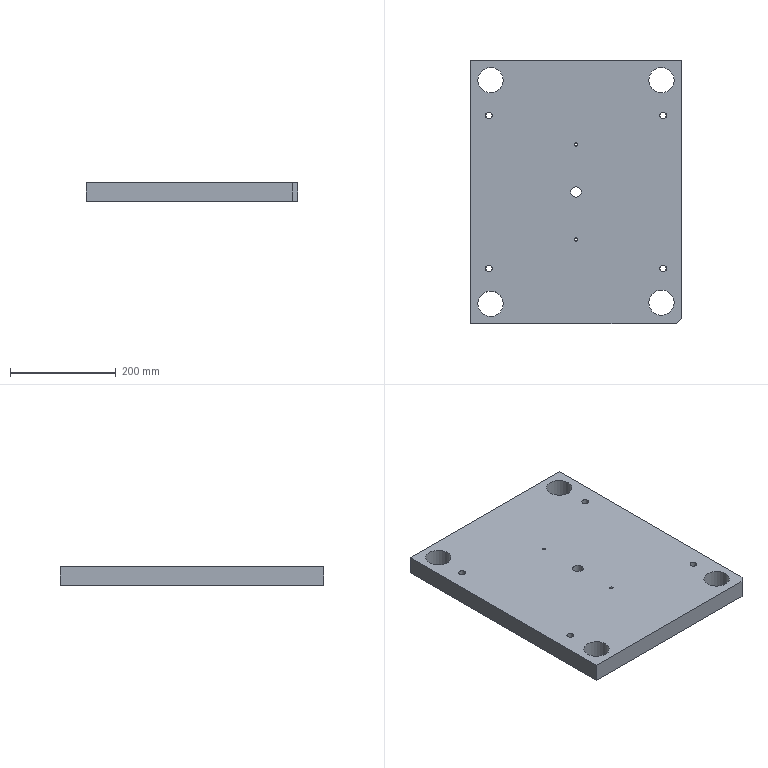Part | STEP file | SL2-MOLD_id726_xmt_txt | 1 solid | 28 faces | box 400 x 500 x 35 mm | volume 6713866 mm3 | cylinder 15 | plane 11 | cone 2 | commonest cylinder face diameters 12 x4 13 x4 48 x4 6 x2 20 x1
STEP:
#1=CARTESIAN_POINT('',(-171.,235.,109.));
#2=VERTEX_POINT('',#1);
#3=CARTESIAN_POINT('',(-165.,235.,109.));
#4=DIRECTION('',(0.,0.,1.));
#5=DIRECTION('',(-1.,0.,0.));
#6=AXIS2_PLACEMENT_3D('',#3,#4,#5);
#7=CIRCLE('',#6,6.);
#8=EDGE_CURVE('',#2,#2,#7,.T.);
#9=ORIENTED_EDGE('',*,*,#8,.F.);
#10=EDGE_LOOP('',(#9));
#11=FACE_BOUND('',#10,.T.);
#12=CARTESIAN_POINT('',(-171.5,235.,109.));
#13=VERTEX_POINT('',#12);
#14=CARTESIAN_POINT('',(-165.,235.,109.));
#15=DIRECTION('',(0.,0.,-1.));
#16=DIRECTION('',(-1.,0.,0.));
#17=AXIS2_PLACEMENT_3D('',#14,#15,#16);
#18=CIRCLE('',#17,6.5);
#19=EDGE_CURVE('',#13,#13,#18,.T.);
#20=ORIENTED_EDGE('',*,*,#19,.F.);
#21=EDGE_LOOP('',(#20));
#22=FACE_BOUND('',#21,.T.);
#23=CARTESIAN_POINT('',(0.,90.,109.));
#24=DIRECTION('',(0.,0.,-1.));
#25=DIRECTION('',(-1.,0.,0.));
#26=AXIS2_PLACEMENT_3D('',#23,#24,#25);
#27=PLANE('',#26);
#28=ADVANCED_FACE('',(#11,#22),#27,.F.);
#29=CARTESIAN_POINT('',(-171.5,-55.,109.));
#30=VERTEX_POINT('',#29);
#31=CARTESIAN_POINT('',(-165.,-55.,109.));
#32=DIRECTION('',(0.,0.,1.));
#33=DIRECTION('',(-1.,0.,0.));
#34=AXIS2_PLACEMENT_3D('',#31,#32,#33);
#35=CIRCLE('',#34,6.5);
#36=EDGE_CURVE('',#30,#30,#35,.T.);
#37=ORIENTED_EDGE('',*,*,#36,.T.);
#38=EDGE_LOOP('',(#37));
#39=FACE_BOUND('',#38,.T.);
#40=CARTESIAN_POINT('',(-171.,-55.,109.));
#41=VERTEX_POINT('',#40);
#42=CARTESIAN_POINT('',(-165.,-55.,109.));
#43=DIRECTION('',(0.,0.,-1.));
#44=DIRECTION('',(-1.,0.,0.));
#45=AXIS2_PLACEMENT_3D('',#42,#43,#44);
#46=CIRCLE('',#45,6.);
#47=EDGE_CURVE('',#41,#41,#46,.T.);
#48=ORIENTED_EDGE('',*,*,#47,.T.);
#49=EDGE_LOOP('',(#48));
#50=FACE_BOUND('',#49,.T.);
#51=CARTESIAN_POINT('',(0.,90.,109.));
#52=DIRECTION('',(0.,0.,-1.));
#53=DIRECTION('',(-1.,0.,0.));
#54=AXIS2_PLACEMENT_3D('',#51,#52,#53);
#55=PLANE('',#54);
#56=ADVANCED_FACE('',(#39,#50),#55,.F.);
#57=CARTESIAN_POINT('',(159.,-55.,109.));
#58=VERTEX_POINT('',#57);
#59=CARTESIAN_POINT('',(165.,-55.,109.));
#60=DIRECTION('',(0.,0.,1.));
#61=DIRECTION('',(-1.,0.,0.));
#62=AXIS2_PLACEMENT_3D('',#59,#60,#61);
#63=CIRCLE('',#62,6.);
#64=EDGE_CURVE('',#58,#58,#63,.T.);
#65=ORIENTED_EDGE('',*,*,#64,.F.);
#66=EDGE_LOOP('',(#65));
#67=FACE_BOUND('',#66,.T.);
#68=CARTESIAN_POINT('',(158.5,-55.,109.));
#69=VERTEX_POINT('',#68);
#70=CARTESIAN_POINT('',(165.,-55.,109.));
#71=DIRECTION('',(0.,0.,-1.));
#72=DIRECTION('',(-1.,0.,0.));
#73=AXIS2_PLACEMENT_3D('',#70,#71,#72);
#74=CIRCLE('',#73,6.5);
#75=EDGE_CURVE('',#69,#69,#74,.T.);
#76=ORIENTED_EDGE('',*,*,#75,.F.);
#77=EDGE_LOOP('',(#76));
#78=FACE_BOUND('',#77,.T.);
#79=CARTESIAN_POINT('',(0.,90.,109.));
#80=DIRECTION('',(0.,0.,-1.));
#81=DIRECTION('',(-1.,0.,0.));
#82=AXIS2_PLACEMENT_3D('',#79,#80,#81);
#83=PLANE('',#82);
#84=ADVANCED_FACE('',(#67,#78),#83,.F.);
#85=CARTESIAN_POINT('',(-159.,235.,101.));
#86=VERTEX_POINT('',#85);
#87=CARTESIAN_POINT('',(-165.,235.,101.));
#88=DIRECTION('',(0.,0.,1.));
#89=DIRECTION('',(1.,0.,0.));
#90=AXIS2_PLACEMENT_3D('',#87,#88,#89);
#91=CIRCLE('',#90,6.);
#92=EDGE_CURVE('',#86,#86,#91,.T.);
#93=ORIENTED_EDGE('',*,*,#92,.T.);
#94=EDGE_LOOP('',(#93));
#95=FACE_BOUND('',#94,.T.);
#96=CARTESIAN_POINT('',(171.,235.,101.));
#97=VERTEX_POINT('',#96);
#98=CARTESIAN_POINT('',(165.,235.,101.));
#99=DIRECTION('',(0.,0.,1.));
#100=DIRECTION('',(1.,0.,0.));
#101=AXIS2_PLACEMENT_3D('',#98,#99,#100);
#102=CIRCLE('',#101,6.);
#103=EDGE_CURVE('',#97,#97,#102,.T.);
#104=ORIENTED_EDGE('',*,*,#103,.T.);
#105=EDGE_LOOP('',(#104));
#106=FACE_BOUND('',#105,.T.);
#107=CARTESIAN_POINT('',(-159.,-55.,101.));
#108=VERTEX_POINT('',#107);
#109=CARTESIAN_POINT('',(-165.,-55.,101.));
#110=DIRECTION('',(0.,0.,1.));
#111=DIRECTION('',(1.,0.,0.));
#112=AXIS2_PLACEMENT_3D('',#109,#110,#111);
#113=CIRCLE('',#112,6.);
#114=EDGE_CURVE('',#108,#108,#113,.T.);
#115=ORIENTED_EDGE('',*,*,#114,.T.);
#116=EDGE_LOOP('',(#115));
#117=FACE_BOUND('',#116,.T.);
#118=CARTESIAN_POINT('',(171.,-55.,101.));
#119=VERTEX_POINT('',#118);
#120=CARTESIAN_POINT('',(165.,-55.,101.));
#121=DIRECTION('',(0.,0.,1.));
#122=DIRECTION('',(1.,0.,0.));
#123=AXIS2_PLACEMENT_3D('',#120,#121,#122);
#124=CIRCLE('',#123,6.);
#125=EDGE_CURVE('',#119,#119,#124,.T.);
#126=ORIENTED_EDGE('',*,*,#125,.T.);
#127=EDGE_LOOP('',(#126));
#128=FACE_BOUND('',#127,.T.);
#129=CARTESIAN_POINT('',(-4.732,0.,101.));
#130=VERTEX_POINT('',#129);
#131=CARTESIAN_POINT('',(0.,0.,101.));
#132=DIRECTION('',(0.,0.,-1.));
#133=DIRECTION('',(-1.,0.,0.));
#134=AXIS2_PLACEMENT_3D('',#131,#132,#133);
#135=CIRCLE('',#134,4.732);
#136=EDGE_CURVE('',#130,#130,#135,.T.);
#137=ORIENTED_EDGE('',*,*,#136,.F.);
#138=EDGE_LOOP('',(#137));
#139=FACE_BOUND('',#138,.T.);
#140=CARTESIAN_POINT('',(-4.732,180.,101.));
#141=VERTEX_POINT('',#140);
#142=CARTESIAN_POINT('',(0.,180.,101.));
#143=DIRECTION('',(0.,0.,-1.));
#144=DIRECTION('',(-1.,0.,0.));
#145=AXIS2_PLACEMENT_3D('',#142,#143,#144);
#146=CIRCLE('',#145,4.732);
#147=EDGE_CURVE('',#141,#141,#146,.T.);
#148=ORIENTED_EDGE('',*,*,#147,.F.);
#149=EDGE_LOOP('',(#148));
#150=FACE_BOUND('',#149,.T.);
#151=CARTESIAN_POINT('',(200.,340.,101.));
#152=VERTEX_POINT('',#151);
#153=CARTESIAN_POINT('',(200.,-150.,101.));
#154=VERTEX_POINT('',#153);
#155=CARTESIAN_POINT('',(200.,-110.,101.));
#156=DIRECTION('',(0.,-1.,0.));
#157=VECTOR('',#156,1.);
#158=LINE('',#155,#157);
#159=EDGE_CURVE('',#152,#154,#158,.T.);
#160=ORIENTED_EDGE('',*,*,#159,.T.);
#161=CARTESIAN_POINT('',(190.,-160.,101.));
#162=VERTEX_POINT('',#161);
#163=CARTESIAN_POINT('',(200.,-150.,101.));
#164=DIRECTION('',(-0.7071,-0.7071,0.));
#165=VECTOR('',#164,1.);
#166=LINE('',#163,#165);
#167=EDGE_CURVE('',#154,#162,#166,.T.);
#168=ORIENTED_EDGE('',*,*,#167,.T.);
#169=CARTESIAN_POINT('',(-200.,-160.,101.));
#170=VERTEX_POINT('',#169);
#171=CARTESIAN_POINT('',(-130.,-160.,101.));
#172=DIRECTION('',(1.,0.,0.));
#173=VECTOR('',#172,1.);
#174=LINE('',#171,#173);
#175=EDGE_CURVE('',#170,#162,#174,.T.);
#176=ORIENTED_EDGE('',*,*,#175,.F.);
#177=CARTESIAN_POINT('',(-200.,340.,101.));
#178=VERTEX_POINT('',#177);
#179=CARTESIAN_POINT('',(-200.,-4.582,101.));
#180=DIRECTION('',(0.,1.,0.));
#181=VECTOR('',#180,1.);
#182=LINE('',#179,#181);
#183=EDGE_CURVE('',#170,#178,#182,.T.);
#184=ORIENTED_EDGE('',*,*,#183,.T.);
#185=CARTESIAN_POINT('',(1.401,340.,101.));
#186=DIRECTION('',(-1.,0.,0.));
#187=VECTOR('',#186,1.);
#188=LINE('',#185,#187);
#189=EDGE_CURVE('',#152,#178,#188,.T.);
#190=ORIENTED_EDGE('',*,*,#189,.F.);
#191=EDGE_LOOP('',(#160,#168,#176,#184,#190));
#192=FACE_BOUND('',#191,.T.);
#193=CARTESIAN_POINT('',(-186.,-122.,101.));
#194=VERTEX_POINT('',#193);
#195=CARTESIAN_POINT('',(-162.,-122.,101.));
#196=DIRECTION('',(0.,0.,1.));
#197=DIRECTION('',(-1.,0.,0.));
#198=AXIS2_PLACEMENT_3D('',#195,#196,#197);
#199=CIRCLE('',#198,24.);
#200=EDGE_CURVE('',#194,#194,#199,.T.);
#201=ORIENTED_EDGE('',*,*,#200,.T.);
#202=EDGE_LOOP('',(#201));
#203=FACE_BOUND('',#202,.T.);
#204=CARTESIAN_POINT('',(138.,-120.,101.));
#205=VERTEX_POINT('',#204);
#206=CARTESIAN_POINT('',(162.,-120.,101.));
#207=DIRECTION('',(0.,0.,1.));
#208=DIRECTION('',(-1.,0.,0.));
#209=AXIS2_PLACEMENT_3D('',#206,#207,#208);
#210=CIRCLE('',#209,24.);
#211=EDGE_CURVE('',#205,#205,#210,.T.);
#212=ORIENTED_EDGE('',*,*,#211,.T.);
#213=EDGE_LOOP('',(#212));
#214=FACE_BOUND('',#213,.T.);
#215=CARTESIAN_POINT('',(-186.,302.,101.));
#216=VERTEX_POINT('',#215);
#217=CARTESIAN_POINT('',(-162.,302.,101.));
#218=DIRECTION('',(0.,0.,1.));
#219=DIRECTION('',(-1.,0.,0.));
#220=AXIS2_PLACEMENT_3D('',#217,#218,#219);
#221=CIRCLE('',#220,24.);
#222=EDGE_CURVE('',#216,#216,#221,.T.);
#223=ORIENTED_EDGE('',*,*,#222,.T.);
#224=EDGE_LOOP('',(#223));
#225=FACE_BOUND('',#224,.T.);
#226=CARTESIAN_POINT('',(138.,302.,101.));
#227=VERTEX_POINT('',#226);
#228=CARTESIAN_POINT('',(162.,302.,101.));
#229=DIRECTION('',(0.,0.,1.));
#230=DIRECTION('',(-1.,0.,0.));
#231=AXIS2_PLACEMENT_3D('',#228,#229,#230);
#232=CIRCLE('',#231,24.);
#233=EDGE_CURVE('',#227,#227,#232,.T.);
#234=ORIENTED_EDGE('',*,*,#233,.T.);
#235=EDGE_LOOP('',(#234));
#236=FACE_BOUND('',#235,.T.);
#237=CARTESIAN_POINT('',(10.,90.,101.));
#238=VERTEX_POINT('',#237);
#239=CARTESIAN_POINT('',(0.,90.,101.));
#240=DIRECTION('',(0.,0.,1.));
#241=DIRECTION('',(1.,0.,0.));
#242=AXIS2_PLACEMENT_3D('',#239,#240,#241);
#243=CIRCLE('',#242,10.);
#244=EDGE_CURVE('',#238,#238,#243,.T.);
#245=ORIENTED_EDGE('',*,*,#244,.T.);
#246=EDGE_LOOP('',(#245));
#247=FACE_BOUND('',#246,.T.);
#248=CARTESIAN_POINT('',(1.401,-4.582,101.));
#249=DIRECTION('',(0.,0.,1.));
#250=DIRECTION('',(1.,0.,0.));
#251=AXIS2_PLACEMENT_3D('',#248,#249,#250);
#252=PLANE('',#251);
#253=ADVANCED_FACE('',(#95,#106,#117,#128,#139,#150,#192,#203,#214,#225,#236,#247),#252,.F.);
#254=CARTESIAN_POINT('',(190.,-160.,136.));
#255=VERTEX_POINT('',#254);
#256=CARTESIAN_POINT('',(190.,-160.,136.));
#257=DIRECTION('',(0.,0.,1.));
#258=VECTOR('',#257,1.);
#259=LINE('',#256,#258);
#260=EDGE_CURVE('',#162,#255,#259,.T.);
#261=ORIENTED_EDGE('',*,*,#260,.T.);
#262=CARTESIAN_POINT('',(-200.,-160.,136.));
#263=VERTEX_POINT('',#262);
#264=CARTESIAN_POINT('',(-130.,-160.,136.));
#265=DIRECTION('',(1.,0.,0.));
#266=VECTOR('',#265,1.);
#267=LINE('',#264,#266);
#268=EDGE_CURVE('',#263,#255,#267,.T.);
#269=ORIENTED_EDGE('',*,*,#268,.F.);
#270=CARTESIAN_POINT('',(-200.,-160.,136.));
#271=DIRECTION('',(0.,0.,-1.));
#272=VECTOR('',#271,1.);
#273=LINE('',#270,#272);
#274=EDGE_CURVE('',#263,#170,#273,.T.);
#275=ORIENTED_EDGE('',*,*,#274,.T.);
#276=ORIENTED_EDGE('',*,*,#175,.T.);
#277=EDGE_LOOP('',(#261,#269,#275,#276));
#278=FACE_OUTER_BOUND('',#277,.T.);
#279=CARTESIAN_POINT('',(-130.,-160.,136.));
#280=DIRECTION('',(0.,1.,0.));
#281=DIRECTION('',(0.,0.,1.));
#282=AXIS2_PLACEMENT_3D('',#279,#280,#281);
#283=PLANE('',#282);
#284=ADVANCED_FACE('',(#278),#283,.F.);
#285=CARTESIAN_POINT('',(200.,340.,136.));
#286=VERTEX_POINT('',#285);
#287=CARTESIAN_POINT('',(200.,340.,136.));
#288=DIRECTION('',(0.,0.,-1.));
#289=VECTOR('',#288,1.);
#290=LINE('',#287,#289);
#291=EDGE_CURVE('',#286,#152,#290,.T.);
#292=ORIENTED_EDGE('',*,*,#291,.F.);
#293=CARTESIAN_POINT('',(200.,-150.,136.));
#294=VERTEX_POINT('',#293);
#295=CARTESIAN_POINT('',(200.,-110.,136.));
#296=DIRECTION('',(0.,-1.,0.));
#297=VECTOR('',#296,1.);
#298=LINE('',#295,#297);
#299=EDGE_CURVE('',#286,#294,#298,.T.);
#300=ORIENTED_EDGE('',*,*,#299,.T.);
#301=CARTESIAN_POINT('',(200.,-150.,101.));
#302=DIRECTION('',(0.,0.,-1.));
#303=VECTOR('',#302,1.);
#304=LINE('',#301,#303);
#305=EDGE_CURVE('',#294,#154,#304,.T.);
#306=ORIENTED_EDGE('',*,*,#305,.T.);
#307=ORIENTED_EDGE('',*,*,#159,.F.);
#308=EDGE_LOOP('',(#292,#300,#306,#307));
#309=FACE_OUTER_BOUND('',#308,.T.);
#310=CARTESIAN_POINT('',(200.,-110.,136.));
#311=DIRECTION('',(1.,0.,0.));
#312=DIRECTION('',(0.,0.,-1.));
#313=AXIS2_PLACEMENT_3D('',#310,#311,#312);
#314=PLANE('',#313);
#315=ADVANCED_FACE('',(#309),#314,.T.);
#316=CARTESIAN_POINT('',(-200.,340.,136.));
#317=VERTEX_POINT('',#316);
#318=CARTESIAN_POINT('',(-200.,340.,136.));
#319=DIRECTION('',(0.,0.,-1.));
#320=VECTOR('',#319,1.);
#321=LINE('',#318,#320);
#322=EDGE_CURVE('',#317,#178,#321,.T.);
#323=ORIENTED_EDGE('',*,*,#322,.F.);
#324=CARTESIAN_POINT('',(1.401,340.,136.));
#325=DIRECTION('',(-1.,0.,0.));
#326=VECTOR('',#325,1.);
#327=LINE('',#324,#326);
#328=EDGE_CURVE('',#286,#317,#327,.T.);
#329=ORIENTED_EDGE('',*,*,#328,.F.);
#330=ORIENTED_EDGE('',*,*,#291,.T.);
#331=ORIENTED_EDGE('',*,*,#189,.T.);
#332=EDGE_LOOP('',(#323,#329,#330,#331));
#333=FACE_OUTER_BOUND('',#332,.T.);
#334=CARTESIAN_POINT('',(1.401,340.,136.));
#335=DIRECTION('',(0.,-1.,0.));
#336=DIRECTION('',(0.,0.,-1.));
#337=AXIS2_PLACEMENT_3D('',#334,#335,#336);
#338=PLANE('',#337);
#339=ADVANCED_FACE('',(#333),#338,.F.);
#340=ORIENTED_EDGE('',*,*,#274,.F.);
#341=CARTESIAN_POINT('',(-200.,-4.582,136.));
#342=DIRECTION('',(0.,1.,0.));
#343=VECTOR('',#342,1.);
#344=LINE('',#341,#343);
#345=EDGE_CURVE('',#263,#317,#344,.T.);
#346=ORIENTED_EDGE('',*,*,#345,.T.);
#347=ORIENTED_EDGE('',*,*,#322,.T.);
#348=ORIENTED_EDGE('',*,*,#183,.F.);
#349=EDGE_LOOP('',(#340,#346,#347,#348));
#350=FACE_OUTER_BOUND('',#349,.T.);
#351=CARTESIAN_POINT('',(-200.,-4.582,136.));
#352=DIRECTION('',(-1.,0.,0.));
#353=DIRECTION('',(0.,0.,1.));
#354=AXIS2_PLACEMENT_3D('',#351,#352,#353);
#355=PLANE('',#354);
#356=ADVANCED_FACE('',(#350),#355,.T.);
#357=ORIENTED_EDGE('',*,*,#305,.F.);
#358=CARTESIAN_POINT('',(173.409,-176.591,136.));
#359=DIRECTION('',(0.7071,0.7071,0.));
#360=VECTOR('',#359,1.);
#361=LINE('',#358,#360);
#362=EDGE_CURVE('',#255,#294,#361,.T.);
#363=ORIENTED_EDGE('',*,*,#362,.F.);
#364=ORIENTED_EDGE('',*,*,#260,.F.);
#365=ORIENTED_EDGE('',*,*,#167,.F.);
#366=EDGE_LOOP('',(#357,#363,#364,#365));
#367=FACE_OUTER_BOUND('',#366,.T.);
#368=CARTESIAN_POINT('',(200.,-150.,136.));
#369=DIRECTION('',(0.7071,-0.7071,0.));
#370=DIRECTION('',(0.,0.,1.));
#371=AXIS2_PLACEMENT_3D('',#368,#369,#370);
#372=PLANE('',#371);
#373=ADVANCED_FACE('',(#367),#372,.T.);
#374=ORIENTED_EDGE('',*,*,#200,.F.);
#375=EDGE_LOOP('',(#374));
#376=FACE_BOUND('',#375,.T.);
#377=CARTESIAN_POINT('',(-138.,-122.,136.));
#378=VERTEX_POINT('',#377);
#379=CARTESIAN_POINT('',(-162.,-122.,136.));
#380=DIRECTION('',(0.,0.,-1.));
#381=DIRECTION('',(1.,0.,0.));
#382=AXIS2_PLACEMENT_3D('',#379,#380,#381);
#383=CIRCLE('',#382,24.);
#384=EDGE_CURVE('',#378,#378,#383,.T.);
#385=ORIENTED_EDGE('',*,*,#384,.F.);
#386=EDGE_LOOP('',(#385));
#387=FACE_BOUND('',#386,.T.);
#388=CARTESIAN_POINT('',(-162.,-122.,149.5));
#389=DIRECTION('',(0.,0.,-1.));
#390=DIRECTION('',(-1.,0.,0.));
#391=AXIS2_PLACEMENT_3D('',#388,#389,#390);
#392=CYLINDRICAL_SURFACE('',#391,24.);
#393=ADVANCED_FACE('',(#376,#387),#392,.F.);
#394=ORIENTED_EDGE('',*,*,#211,.F.);
#395=EDGE_LOOP('',(#394));
#396=FACE_BOUND('',#395,.T.);
#397=CARTESIAN_POINT('',(186.,-120.,136.));
#398=VERTEX_POINT('',#397);
#399=CARTESIAN_POINT('',(162.,-120.,136.));
#400=DIRECTION('',(0.,0.,-1.));
#401=DIRECTION('',(1.,0.,0.));
#402=AXIS2_PLACEMENT_3D('',#399,#400,#401);
#403=CIRCLE('',#402,24.);
#404=EDGE_CURVE('',#398,#398,#403,.T.);
#405=ORIENTED_EDGE('',*,*,#404,.F.);
#406=EDGE_LOOP('',(#405));
#407=FACE_BOUND('',#406,.T.);
#408=CARTESIAN_POINT('',(162.,-120.,149.5));
#409=DIRECTION('',(0.,0.,-1.));
#410=DIRECTION('',(-1.,0.,0.));
#411=AXIS2_PLACEMENT_3D('',#408,#409,#410);
#412=CYLINDRICAL_SURFACE('',#411,24.);
#413=ADVANCED_FACE('',(#396,#407),#412,.F.);
#414=ORIENTED_EDGE('',*,*,#222,.F.);
#415=EDGE_LOOP('',(#414));
#416=FACE_BOUND('',#415,.T.);
#417=CARTESIAN_POINT('',(-138.,302.,136.));
#418=VERTEX_POINT('',#417);
#419=CARTESIAN_POINT('',(-162.,302.,136.));
#420=DIRECTION('',(0.,0.,-1.));
#421=DIRECTION('',(1.,0.,0.));
#422=AXIS2_PLACEMENT_3D('',#419,#420,#421);
#423=CIRCLE('',#422,24.);
#424=EDGE_CURVE('',#418,#418,#423,.T.);
#425=ORIENTED_EDGE('',*,*,#424,.F.);
#426=EDGE_LOOP('',(#425));
#427=FACE_BOUND('',#426,.T.);
#428=CARTESIAN_POINT('',(-162.,302.,149.5));
#429=DIRECTION('',(0.,0.,-1.));
#430=DIRECTION('',(-1.,0.,0.));
#431=AXIS2_PLACEMENT_3D('',#428,#429,#430);
#432=CYLINDRICAL_SURFACE('',#431,24.);
#433=ADVANCED_FACE('',(#416,#427),#432,.F.);
#434=ORIENTED_EDGE('',*,*,#233,.F.);
#435=EDGE_LOOP('',(#434));
#436=FACE_BOUND('',#435,.T.);
#437=CARTESIAN_POINT('',(186.,302.,136.));
#438=VERTEX_POINT('',#437);
#439=CARTESIAN_POINT('',(162.,302.,136.));
#440=DIRECTION('',(0.,0.,-1.));
#441=DIRECTION('',(1.,0.,0.));
#442=AXIS2_PLACEMENT_3D('',#439,#440,#441);
#443=CIRCLE('',#442,24.);
#444=EDGE_CURVE('',#438,#438,#443,.T.);
#445=ORIENTED_EDGE('',*,*,#444,.F.);
#446=EDGE_LOOP('',(#445));
#447=FACE_BOUND('',#446,.T.);
#448=CARTESIAN_POINT('',(162.,302.,149.5));
#449=DIRECTION('',(0.,0.,-1.));
#450=DIRECTION('',(-1.,0.,0.));
#451=AXIS2_PLACEMENT_3D('',#448,#449,#450);
#452=CYLINDRICAL_SURFACE('',#451,24.);
#453=ADVANCED_FACE('',(#436,#447),#452,.F.);
#454=ORIENTED_EDGE('',*,*,#244,.F.);
#455=EDGE_LOOP('',(#454));
#456=FACE_BOUND('',#455,.T.);
#457=CARTESIAN_POINT('',(10.,90.,136.));
#458=VERTEX_POINT('',#457);
#459=CARTESIAN_POINT('',(0.,90.,136.));
#460=DIRECTION('',(0.,0.,1.));
#461=DIRECTION('',(1.,0.,0.));
#462=AXIS2_PLACEMENT_3D('',#459,#460,#461);
#463=CIRCLE('',#462,10.);
#464=EDGE_CURVE('',#458,#458,#463,.T.);
#465=ORIENTED_EDGE('',*,*,#464,.T.);
#466=EDGE_LOOP('',(#465));
#467=FACE_BOUND('',#466,.T.);
#468=CARTESIAN_POINT('',(0.,90.,145.615));
#469=DIRECTION('',(0.,0.,1.));
#470=DIRECTION('',(0.,-1.,0.));
#471=AXIS2_PLACEMENT_3D('',#468,#469,#470);
#472=CYLINDRICAL_SURFACE('',#471,10.);
#473=ADVANCED_FACE('',(#456,#467),#472,.F.);
#474=CARTESIAN_POINT('',(-3.,0.,104.));
#475=VERTEX_POINT('',#474);
#476=CARTESIAN_POINT('',(0.,0.,104.));
#477=DIRECTION('',(0.,0.,-1.));
#478=DIRECTION('',(-1.,0.,0.));
#479=AXIS2_PLACEMENT_3D('',#476,#477,#478);
#480=CIRCLE('',#479,3.);
#481=EDGE_CURVE('',#475,#475,#480,.T.);
#482=ORIENTED_EDGE('',*,*,#481,.T.);
#483=EDGE_LOOP('',(#482));
#484=FACE_BOUND('',#483,.T.);
#485=CARTESIAN_POINT('',(3.,0.,136.));
#486=VERTEX_POINT('',#485);
#487=CARTESIAN_POINT('',(0.,0.,136.));
#488=DIRECTION('',(0.,0.,-1.));
#489=DIRECTION('',(1.,0.,0.));
#490=AXIS2_PLACEMENT_3D('',#487,#488,#489);
#491=CIRCLE('',#490,3.);
#492=EDGE_CURVE('',#486,#486,#491,.T.);
#493=ORIENTED_EDGE('',*,*,#492,.F.);
#494=EDGE_LOOP('',(#493));
#495=FACE_BOUND('',#494,.T.);
#496=CARTESIAN_POINT('',(0.,0.,658.4));
#497=DIRECTION('',(0.,0.,-1.));
#498=DIRECTION('',(-1.,0.,0.));
#499=AXIS2_PLACEMENT_3D('',#496,#497,#498);
#500=CYLINDRICAL_SURFACE('',#499,3.);
#501=ADVANCED_FACE('',(#484,#495),#500,.F.);
#502=CARTESIAN_POINT('',(-3.,180.,104.));
#503=VERTEX_POINT('',#502);
#504=CARTESIAN_POINT('',(0.,180.,104.));
#505=DIRECTION('',(0.,0.,-1.));
#506=DIRECTION('',(-1.,0.,0.));
#507=AXIS2_PLACEMENT_3D('',#504,#505,#506);
#508=CIRCLE('',#507,3.);
#509=EDGE_CURVE('',#503,#503,#508,.T.);
#510=ORIENTED_EDGE('',*,*,#509,.T.);
#511=EDGE_LOOP('',(#510));
#512=FACE_BOUND('',#511,.T.);
#513=CARTESIAN_POINT('',(3.,180.,136.));
#514=VERTEX_POINT('',#513);
#515=CARTESIAN_POINT('',(0.,180.,136.));
#516=DIRECTION('',(0.,0.,-1.));
#517=DIRECTION('',(1.,0.,0.));
#518=AXIS2_PLACEMENT_3D('',#515,#516,#517);
#519=CIRCLE('',#518,3.);
#520=EDGE_CURVE('',#514,#514,#519,.T.);
#521=ORIENTED_EDGE('',*,*,#520,.F.);
#522=EDGE_LOOP('',(#521));
#523=FACE_BOUND('',#522,.T.);
#524=CARTESIAN_POINT('',(0.,180.,658.4));
#525=DIRECTION('',(0.,0.,-1.));
#526=DIRECTION('',(-1.,0.,0.));
#527=AXIS2_PLACEMENT_3D('',#524,#525,#526);
#528=CYLINDRICAL_SURFACE('',#527,3.);
#529=ADVANCED_FACE('',(#512,#523),#528,.F.);
#530=ORIENTED_EDGE('',*,*,#509,.F.);
#531=EDGE_LOOP('',(#530));
#532=FACE_BOUND('',#531,.T.);
#533=ORIENTED_EDGE('',*,*,#147,.T.);
#534=EDGE_LOOP('',(#533));
#535=FACE_BOUND('',#534,.T.);
#536=CARTESIAN_POINT('',(0.,180.,104.));
#537=DIRECTION('',(0.,0.,-1.));
#538=DIRECTION('',(-1.,0.,0.));
#539=AXIS2_PLACEMENT_3D('',#536,#537,#538);
#540=CONICAL_SURFACE('',#539,3.,30.);
#541=ADVANCED_FACE('',(#532,#535),#540,.F.);
#542=ORIENTED_EDGE('',*,*,#481,.F.);
#543=EDGE_LOOP('',(#542));
#544=FACE_BOUND('',#543,.T.);
#545=ORIENTED_EDGE('',*,*,#136,.T.);
#546=EDGE_LOOP('',(#545));
#547=FACE_BOUND('',#546,.T.);
#548=CARTESIAN_POINT('',(0.,0.,104.));
#549=DIRECTION('',(0.,0.,-1.));
#550=DIRECTION('',(-1.,0.,0.));
#551=AXIS2_PLACEMENT_3D('',#548,#549,#550);
#552=CONICAL_SURFACE('',#551,3.,30.);
#553=ADVANCED_FACE('',(#544,#547),#552,.F.);
#554=ORIENTED_EDGE('',*,*,#64,.T.);
#555=EDGE_LOOP('',(#554));
#556=FACE_BOUND('',#555,.T.);
#557=ORIENTED_EDGE('',*,*,#125,.F.);
#558=EDGE_LOOP('',(#557));
#559=FACE_BOUND('',#558,.T.);
#560=CARTESIAN_POINT('',(165.,-55.,112.));
#561=DIRECTION('',(0.,0.,-1.));
#562=DIRECTION('',(1.,0.,0.));
#563=AXIS2_PLACEMENT_3D('',#560,#561,#562);
#564=CYLINDRICAL_SURFACE('',#563,6.);
#565=ADVANCED_FACE('',(#556,#559),#564,.F.);
#566=ORIENTED_EDGE('',*,*,#47,.F.);
#567=EDGE_LOOP('',(#566));
#568=FACE_BOUND('',#567,.T.);
#569=ORIENTED_EDGE('',*,*,#114,.F.);
#570=EDGE_LOOP('',(#569));
#571=FACE_BOUND('',#570,.T.);
#572=CARTESIAN_POINT('',(-165.,-55.,112.));
#573=DIRECTION('',(0.,0.,-1.));
#574=DIRECTION('',(1.,0.,0.));
#575=AXIS2_PLACEMENT_3D('',#572,#573,#574);
#576=CYLINDRICAL_SURFACE('',#575,6.);
#577=ADVANCED_FACE('',(#568,#571),#576,.F.);
#578=CARTESIAN_POINT('',(159.,235.,109.));
#579=VERTEX_POINT('',#578);
#580=CARTESIAN_POINT('',(165.,235.,109.));
#581=DIRECTION('',(0.,0.,-1.));
#582=DIRECTION('',(-1.,0.,0.));
#583=AXIS2_PLACEMENT_3D('',#580,#581,#582);
#584=CIRCLE('',#583,6.);
#585=EDGE_CURVE('',#579,#579,#584,.T.);
#586=ORIENTED_EDGE('',*,*,#585,.F.);
#587=EDGE_LOOP('',(#586));
#588=FACE_BOUND('',#587,.T.);
#589=ORIENTED_EDGE('',*,*,#103,.F.);
#590=EDGE_LOOP('',(#589));
#591=FACE_BOUND('',#590,.T.);
#592=CARTESIAN_POINT('',(165.,235.,112.));
#593=DIRECTION('',(0.,0.,-1.));
#594=DIRECTION('',(1.,0.,0.));
#595=AXIS2_PLACEMENT_3D('',#592,#593,#594);
#596=CYLINDRICAL_SURFACE('',#595,6.);
#597=ADVANCED_FACE('',(#588,#591),#596,.F.);
#598=ORIENTED_EDGE('',*,*,#8,.T.);
#599=EDGE_LOOP('',(#598));
#600=FACE_BOUND('',#599,.T.);
#601=ORIENTED_EDGE('',*,*,#92,.F.);
#602=EDGE_LOOP('',(#601));
#603=FACE_BOUND('',#602,.T.);
#604=CARTESIAN_POINT('',(-165.,235.,112.));
#605=DIRECTION('',(0.,0.,-1.));
#606=DIRECTION('',(1.,0.,0.));
#607=AXIS2_PLACEMENT_3D('',#604,#605,#606);
#608=CYLINDRICAL_SURFACE('',#607,6.);
#609=ADVANCED_FACE('',(#600,#603),#608,.F.);
#610=CARTESIAN_POINT('',(158.5,235.,109.));
#611=VERTEX_POINT('',#610);
#612=CARTESIAN_POINT('',(165.,235.,109.));
#613=DIRECTION('',(0.,0.,1.));
#614=DIRECTION('',(-1.,0.,0.));
#615=AXIS2_PLACEMENT_3D('',#612,#613,#614);
#616=CIRCLE('',#615,6.5);
#617=EDGE_CURVE('',#611,#611,#616,.T.);
#618=ORIENTED_EDGE('',*,*,#617,.T.);
#619=EDGE_LOOP('',(#618));
#620=FACE_BOUND('',#619,.T.);
#621=ORIENTED_EDGE('',*,*,#585,.T.);
#622=EDGE_LOOP('',(#621));
#623=FACE_BOUND('',#622,.T.);
#624=CARTESIAN_POINT('',(0.,90.,109.));
#625=DIRECTION('',(0.,0.,-1.));
#626=DIRECTION('',(-1.,0.,0.));
#627=AXIS2_PLACEMENT_3D('',#624,#625,#626);
#628=PLANE('',#627);
#629=ADVANCED_FACE('',(#620,#623),#628,.F.);
#630=CARTESIAN_POINT('',(171.5,-55.,136.));
#631=VERTEX_POINT('',#630);
#632=CARTESIAN_POINT('',(165.,-55.,136.));
#633=DIRECTION('',(0.,0.,1.));
#634=DIRECTION('',(1.,0.,0.));
#635=AXIS2_PLACEMENT_3D('',#632,#633,#634);
#636=CIRCLE('',#635,6.5);
#637=EDGE_CURVE('',#631,#631,#636,.T.);
#638=ORIENTED_EDGE('',*,*,#637,.T.);
#639=EDGE_LOOP('',(#638));
#640=FACE_BOUND('',#639,.T.);
#641=ORIENTED_EDGE('',*,*,#75,.T.);
#642=EDGE_LOOP('',(#641));
#643=FACE_BOUND('',#642,.T.);
#644=CARTESIAN_POINT('',(165.,-55.,112.));
#645=DIRECTION('',(0.,0.,-1.));
#646=DIRECTION('',(1.,0.,0.));
#647=AXIS2_PLACEMENT_3D('',#644,#645,#646);
#648=CYLINDRICAL_SURFACE('',#647,6.5);
#649=ADVANCED_FACE('',(#640,#643),#648,.F.);
#650=CARTESIAN_POINT('',(-158.5,-55.,136.));
#651=VERTEX_POINT('',#650);
#652=CARTESIAN_POINT('',(-165.,-55.,136.));
#653=DIRECTION('',(0.,0.,1.));
#654=DIRECTION('',(1.,0.,0.));
#655=AXIS2_PLACEMENT_3D('',#652,#653,#654);
#656=CIRCLE('',#655,6.5);
#657=EDGE_CURVE('',#651,#651,#656,.T.);
#658=ORIENTED_EDGE('',*,*,#657,.T.);
#659=EDGE_LOOP('',(#658));
#660=FACE_BOUND('',#659,.T.);
#661=ORIENTED_EDGE('',*,*,#36,.F.);
#662=EDGE_LOOP('',(#661));
#663=FACE_BOUND('',#662,.T.);
#664=CARTESIAN_POINT('',(-165.,-55.,112.));
#665=DIRECTION('',(0.,0.,-1.));
#666=DIRECTION('',(1.,0.,0.));
#667=AXIS2_PLACEMENT_3D('',#664,#665,#666);
#668=CYLINDRICAL_SURFACE('',#667,6.5);
#669=ADVANCED_FACE('',(#660,#663),#668,.F.);
#670=CARTESIAN_POINT('',(171.5,235.,136.));
#671=VERTEX_POINT('',#670);
#672=CARTESIAN_POINT('',(165.,235.,136.));
#673=DIRECTION('',(0.,0.,1.));
#674=DIRECTION('',(1.,0.,0.));
#675=AXIS2_PLACEMENT_3D('',#672,#673,#674);
#676=CIRCLE('',#675,6.5);
#677=EDGE_CURVE('',#671,#671,#676,.T.);
#678=ORIENTED_EDGE('',*,*,#677,.T.);
#679=EDGE_LOOP('',(#678));
#680=FACE_BOUND('',#679,.T.);
#681=ORIENTED_EDGE('',*,*,#617,.F.);
#682=EDGE_LOOP('',(#681));
#683=FACE_BOUND('',#682,.T.);
#684=CARTESIAN_POINT('',(165.,235.,112.));
#685=DIRECTION('',(0.,0.,-1.));
#686=DIRECTION('',(1.,0.,0.));
#687=AXIS2_PLACEMENT_3D('',#684,#685,#686);
#688=CYLINDRICAL_SURFACE('',#687,6.5);
#689=ADVANCED_FACE('',(#680,#683),#688,.F.);
#690=CARTESIAN_POINT('',(-158.5,235.,136.));
#691=VERTEX_POINT('',#690);
#692=CARTESIAN_POINT('',(-165.,235.,136.));
#693=DIRECTION('',(0.,0.,1.));
#694=DIRECTION('',(1.,0.,0.));
#695=AXIS2_PLACEMENT_3D('',#692,#693,#694);
#696=CIRCLE('',#695,6.5);
#697=EDGE_CURVE('',#691,#691,#696,.T.);
#698=ORIENTED_EDGE('',*,*,#697,.F.);
#699=EDGE_LOOP('',(#698));
#700=FACE_BOUND('',#699,.T.);
#701=ORIENTED_EDGE('',*,*,#677,.F.);
#702=EDGE_LOOP('',(#701));
#703=FACE_BOUND('',#702,.T.);
#704=ORIENTED_EDGE('',*,*,#657,.F.);
#705=EDGE_LOOP('',(#704));
#706=FACE_BOUND('',#705,.T.);
#707=ORIENTED_EDGE('',*,*,#637,.F.);
#708=EDGE_LOOP('',(#707));
#709=FACE_BOUND('',#708,.T.);
#710=ORIENTED_EDGE('',*,*,#520,.T.);
#711=EDGE_LOOP('',(#710));
#712=FACE_BOUND('',#711,.T.);
#713=ORIENTED_EDGE('',*,*,#492,.T.);
#714=EDGE_LOOP('',(#713));
#715=FACE_BOUND('',#714,.T.);
#716=ORIENTED_EDGE('',*,*,#464,.F.);
#717=EDGE_LOOP('',(#716));
#718=FACE_BOUND('',#717,.T.);
#719=ORIENTED_EDGE('',*,*,#444,.T.);
#720=EDGE_LOOP('',(#719));
#721=FACE_BOUND('',#720,.T.);
#722=ORIENTED_EDGE('',*,*,#424,.T.);
#723=EDGE_LOOP('',(#722));
#724=FACE_BOUND('',#723,.T.);
#725=ORIENTED_EDGE('',*,*,#404,.T.);
#726=EDGE_LOOP('',(#725));
#727=FACE_BOUND('',#726,.T.);
#728=ORIENTED_EDGE('',*,*,#384,.T.);
#729=EDGE_LOOP('',(#728));
#730=FACE_BOUND('',#729,.T.);
#731=ORIENTED_EDGE('',*,*,#268,.T.);
#732=ORIENTED_EDGE('',*,*,#362,.T.);
#733=ORIENTED_EDGE('',*,*,#299,.F.);
#734=ORIENTED_EDGE('',*,*,#328,.T.);
#735=ORIENTED_EDGE('',*,*,#345,.F.);
#736=EDGE_LOOP('',(#731,#732,#733,#734,#735));
#737=FACE_BOUND('',#736,.T.);
#738=CARTESIAN_POINT('',(1.401,-4.582,136.));
#739=DIRECTION('',(0.,0.,1.));
#740=DIRECTION('',(1.,0.,0.));
#741=AXIS2_PLACEMENT_3D('',#738,#739,#740);
#742=PLANE('',#741);
#743=ADVANCED_FACE('',(#700,#703,#706,#709,#712,#715,#718,#721,#724,#727,#730,#737),#742,.T.);
#744=ORIENTED_EDGE('',*,*,#697,.T.);
#745=EDGE_LOOP('',(#744));
#746=FACE_BOUND('',#745,.T.);
#747=ORIENTED_EDGE('',*,*,#19,.T.);
#748=EDGE_LOOP('',(#747));
#749=FACE_BOUND('',#748,.T.);
#750=CARTESIAN_POINT('',(-165.,235.,112.));
#751=DIRECTION('',(0.,0.,-1.));
#752=DIRECTION('',(1.,0.,0.));
#753=AXIS2_PLACEMENT_3D('',#750,#751,#752);
#754=CYLINDRICAL_SURFACE('',#753,6.5);
#755=ADVANCED_FACE('',(#746,#749),#754,.F.);
#756=CLOSED_SHELL('',(#28,#56,#84,#253,#284,#315,#339,#356,#373,#393,#413,#433,#453,#473,#501,#529,#541,#553,#565,#577,#597,#609,#629,#649,#669,#689,#743,#755));
#757=MANIFOLD_SOLID_BREP('',#756);
#758=(LENGTH_UNIT()NAMED_UNIT(*)SI_UNIT(.MILLI.,.METRE.));
#759=UNCERTAINTY_MEASURE_WITH_UNIT(LENGTH_MEASURE(0.00002),#758,'','');
#760=(NAMED_UNIT(*)PLANE_ANGLE_UNIT()SI_UNIT($,.RADIAN.));
#761=PLANE_ANGLE_MEASURE_WITH_UNIT(PLANE_ANGLE_MEASURE(0.01745),#760);
#762=DIMENSIONAL_EXPONENTS(0.,0.,0.,0.,0.,0.,0.);
#763=(CONVERSION_BASED_UNIT('DEGREE',#761)NAMED_UNIT(#762)PLANE_ANGLE_UNIT());
#764=(NAMED_UNIT(*)SI_UNIT($,.STERADIAN.)SOLID_ANGLE_UNIT());
#765=(GEOMETRIC_REPRESENTATION_CONTEXT(3)GLOBAL_UNCERTAINTY_ASSIGNED_CONTEXT((#759))GLOBAL_UNIT_ASSIGNED_CONTEXT((#758,#763,#764))REPRESENTATION_CONTEXT('',''));
#766=ADVANCED_BREP_SHAPE_REPRESENTATION('',(#757),#765);